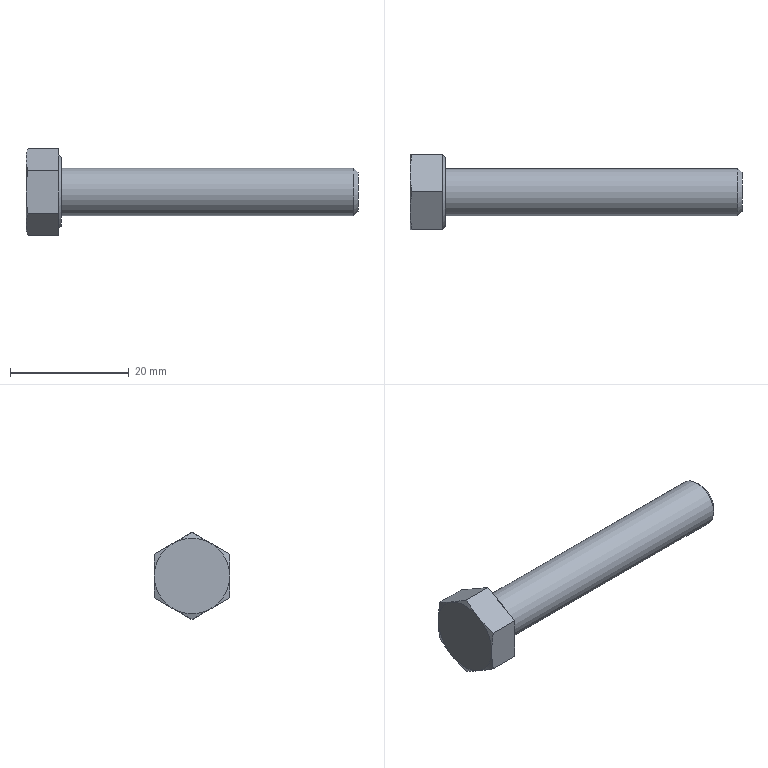Part | STEP file | Hex head bolt M8X50 A2-70 GBT5782-2016_GB_FASTENER_BOLT_SB A M8X40-C | 1 solid | 24 faces | box 55.95 x 12.73 x 14.699 mm | volume 3330 mm3 | plane 15 | cone 8 | cylinder 1 | commonest cylinder face diameters 8 x1